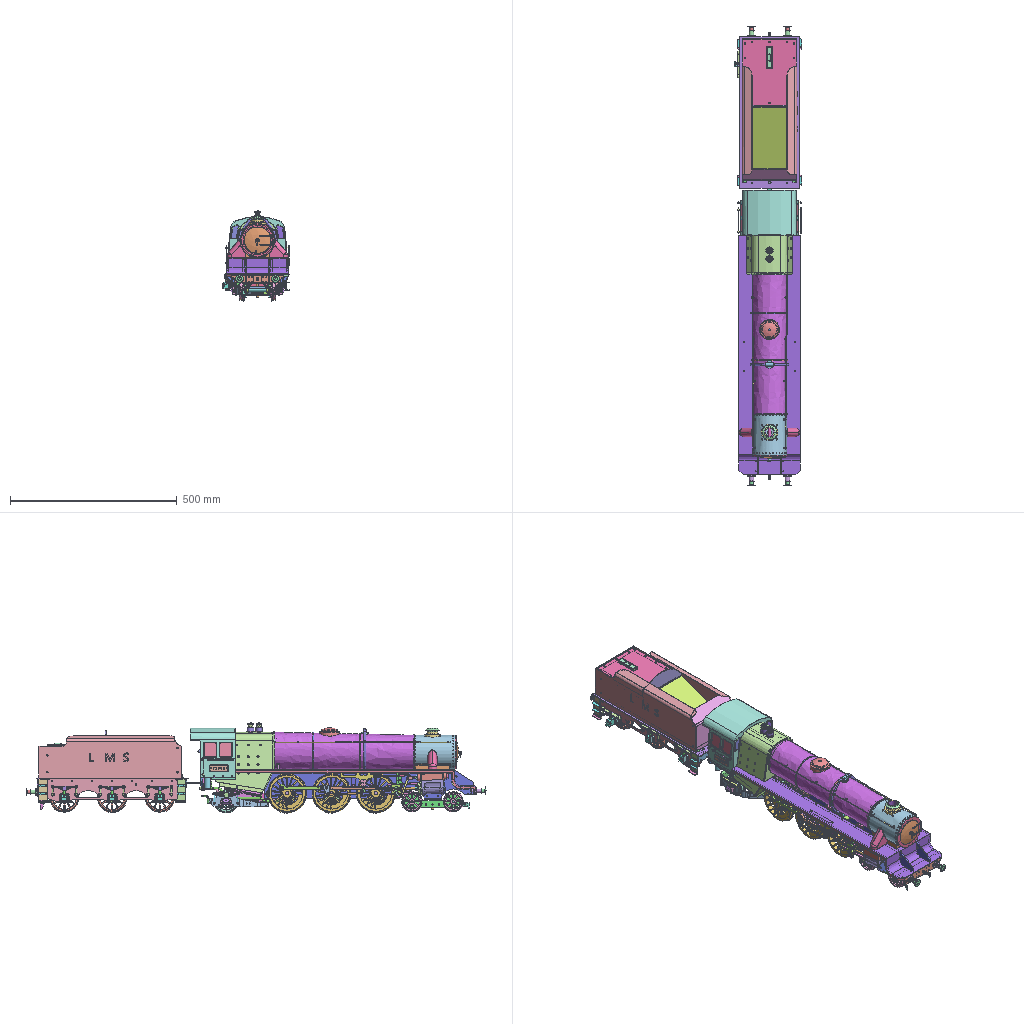Assembly | STEP file | 318 different items | 619 placed | box 202 x 1378 x 271 mm
Parts list (item | name | quantity | parent item | size | volume):
1 | 1-01.14 | x1 | in 1-01 part | 10 x 10 x 33 mm | 1037 mm3
2 | 1-01.13 | x2 | in 1-01 part | 26 x 12 x 30 mm | 2499 mm3
3 | 1-01.12 | x1 | in 1-01 part | 13 x 67 x 13 mm | 5525 mm3
4 | 1-01.11 | x1 | in 1-01 part | 20 x 20 x 1 mm | 235.619 mm3
5 | 1-01.10 | x1 | in 1-01 part | 14.501 x 14.501 x 19.996 mm | 434.428 mm3
6 | 1-01.9 | x1 | in 1-01 part | 10 x 10 x 41 mm | 2711 mm3
7 | 1-01.8 | x2 | in 1-01 part | 51 x 12 x 12 mm | 2118 mm3
8 | 1-01.7 | x1 | in 1-01 part | 51 x 73 x 3 mm | 10792 mm3
9 | 1-01.6 | x1 | in 1-01 part | 16 x 67 x 38 mm | 16896 mm3
10 | 1-01.5 | x2 | in 1-01 part | 21 x 21 x 21 mm | 2287 mm3
11 | 1-01.4 symmetric part | x1 | in 1-01 part | 577.1 x 8 x 56 mm | 13016 mm3
12 | 1-01.4 | x1 | in 1-01 part | 577.1 x 8 x 56 mm | 13016 mm3
13 | 1-01.3 | x1 | in 1-01 part | 12 x 67 x 25 mm | 18121 mm3
14 | 1-01.2 | x1 | in 1-01 part | 25 x 152 x 25 mm | 25515 mm3
15 | 1-01.1 | x2 | in 1-01 part | 3 x 625 x 82.5 mm | 131350 mm3
16 | 1-02 | x6 | in Locomotive assembly | 13 x 50 x 13 mm | 2573 mm3
17 | 1-03.1 | x6 | in 1-03 part | 10 x 25 x 25 mm | 4620 mm3
18 | 1-03.2 | x6 | in 1-03 part | 3 x 3 x 39 mm | 275.675 mm3
19 | 1-03.3 | x6 | in 1-03 part | 5.252 x 5.25 x 22.544 mm | 75.49 mm3
20 | 1-03.4 | x6 | in 1-03 part | 6 x 6 x 1 mm | 21.206 mm3
21 | 1-04.1 | x2 | in 1-04 part | 3 x 173.195 x 38 mm | 12978 mm3
22 | 1-04.2 | x1 | in 1-04 part | 50 x 68 x 12 mm | 11705 mm3
23 | 1-04.3 | x2 | in 1-04 part | 7 x 68 x 7 mm | 2391 mm3
24 | 1-04.4 | x4 | in 1-04 part | 19 x 13 x 19 mm | 1368 mm3
25 | 1-04.5 | x1 | in 1-04 part | 11 x 30 x 17.5 mm | 723.407 mm3
26 | 1-04.5 symmetric part | x1 | in 1-04 part | 11 x 30 x 17.5 mm | 723.407 mm3
27 | 1-05 | x1 | in Locomotive assembly | 106 x 78.066 x 28.5 mm | 78441 mm3
28 | 1-06.1 | x2 | in 1-06 part, 1-06 symmetric subassembly | 64 x 54.5 x 45 mm | 79802 mm3
29 | 1-06.2 | x2 | in 1-06 part, 1-06 symmetric subassembly | 28 x 64 x 28 mm | 7900 mm3
30 | 1-06.3 | x2 | in 1-06 part, 1-06 symmetric subassembly | 13.856 x 12 x 12 mm | 1127 mm3
31 | 1-06.4 | x2 | in 1-06 part, 1-06 symmetric subassembly | 13.856 x 11.5 x 12 mm | 920.282 mm3
32 | 1-06.5 | x2 | in 1-06 part, 1-06 symmetric subassembly | 8 x 4.5 x 8 mm | 169.646 mm3
33 | 1-06.6 | x2 | in 1-06 part, 1-06 symmetric subassembly | 8 x 5.5 x 8 mm | 119.381 mm3
34 | 1-06.7 | x2 | in 1-06 part, 1-06 symmetric subassembly | 45 x 64 x 3 mm | 8287 mm3
35 | 1-06.8 | x2 | in 1-06 part, 1-06 symmetric subassembly | 54.5 x 88 x 23 mm | 33301 mm3
36 | 1-07 | x2 | in Locomotive assembly | 6.5 x 45 x 45 mm | 8285 mm3
37 | 1-08.1 | x2 | in 1-08 part | 13.5 x 45 x 45 mm | 10498 mm3
38 | 1-08.2 | x4 | in 1-08 part | 101 x 6 x 5 mm | 2812 mm3
39 | 1-08.3 | x2 | in 1-08 part | 13.5 x 18.475 x 16 mm | 1580 mm3
40 | 1-08.4 | x2 | in 1-08 part | 4 x 10 x 10 mm | 201.062 mm3
41 | 1-08.5 | x2 | in 1-08 part | 4 x 10 x 10 mm | 144.513 mm3
42 | 1-09.1 | x1 | in Locomotive assembly | 24 x 38 x 77 mm | 9451 mm3
43 | 1-09.1 symmetric part | x1 | in Locomotive assembly | 24 x 38 x 77 mm | 9451 mm3
44 | 1-11.1 | x1 | in 1-11 part | 25 x 40 x 48 mm | 7483 mm3
45 | 1-11.2 | x1 | in 1-11 part | 15 x 17.321 x 16 mm | 1681 mm3
46 | 1-11.3 | x2 | in 1-11 part | 8 x 38 x 8 mm | 835.664 mm3
47 | 1-11.4 | x2 | in 1-11 part | 13.856 x 4 x 12 mm | 297.769 mm3
48 | 1-12.1 | x1 | in 1-12 part | 25 x 14 x 70 mm | 4367 mm3
49 | 1-12.2 | x2 | in 1-12 part | 38 x 10 x 10 mm | 1074 mm3
50 | 1-12.3 | x2 | in 1-12 part | 4 x 16.166 x 14 mm | 364.805 mm3
51 | 1-12.4 | x1 | in 1-12 part | 10 x 11.547 x 13 mm | 537.367 mm3
52 | 1-14.1 | x1 | in 1-14 part | 50.002 x 50.001 x 27 mm | 7555 mm3
53 | 1-14.2 | x1 | in 1-14 part | 36 x 36 x 64.039 mm | 7996 mm3
54 | 1-14.3 | x1 | in 1-14 part | 44 x 44 x 9.5 mm | 3548 mm3
55 | 1-15 | x1 | in Locomotive assembly | 60.001 x 60 x 25.516 mm | 4981 mm3
56 | 1-16.1 | x2 | in 1-16 part | 12 x 12 x 4 mm | 306.305 mm3
57 | 1-16.2 | x2 | in 1-16 part | 16 x 16 x 19 mm | 1038 mm3
58 | 1-16.3 | x2 | in 1-16 part | 4.501 x 4.5 x 11.798 mm | 24.723 mm3
59 | 1-16.4 | x2 | in 1-16 part | 6 x 6 x 20 mm | 175.087 mm3
60 | 1-16.5 | x2 | in 1-16 part | 6 x 6 x 6 mm | 113.097 mm3
61 | 1-16.6 | x2 | in 1-16 part | 19 x 19 x 20 mm | 2980 mm3
62 | 1-23.1 | x1 | in 1-23 part | 37 x 32 x 32 mm | 6942 mm3
63 | 1-23.2 | x1 | in 1-23 part | 142 x 14 x 14 mm | 14676 mm3
64 | 1-23.3 | x1 | in 1-23 part | 21 x 14 x 14 mm | 1943 mm3
65 | 1-23.4 | x1 | in 1-23 part | 427 x 10 x 10 mm | 20870 mm3
66 | 1-23.5 | x1 | in 1-23 part | 185.5 x 10 x 10 mm | 6004 mm3
67 | 1-23.6 | x1 | in 1-23 part | 14 x 17.321 x 15 mm | 1648 mm3
68 | 1-23.7 | x1 | in 1-23 part | 24.52 x 10 x 38.054 mm | 795.308 mm3
69 | 1-26.1 | x1 | in 1-26 part | 8 x 315 x 31 mm | 5686 mm3
70 | 1-26.2 | x1 | in 1-26 part | 8 x 392.074 x 38.526 mm | 7072 mm3
71 | 1-26.3 | x1 | in 1-26 part | 7 x 12 x 22 mm | 969.173 mm3
72 | 1-26.4 | x1 | in 1-26 part | 3 x 12 x 22 mm | 652.172 mm3
73 | 1-28.1 | x1 | in 1-28 part | 184 x 821 x 50 mm | 191096 mm3
74 | 1-28.2 | x1 | in 1-28 part | 716 x 16 x 54 mm | 8341 mm3
75 | 1-28.2 symmetric part | x1 | in 1-28 part | 716 x 16 x 54 mm | 8341 mm3
76 | 1-28.3 | x1 | in 1-28 part | 5 x 172 x 24 mm | 17032 mm3
77 | 1-28.4 | x1 | in 1-28 part | 22 x 110 x 15 mm | 4787 mm3
78 | 1-28.5 | x2 | in 1-28 part | 32 x 5 x 20.5 mm | 1373 mm3
79 | 1-28.6 | x1 | in 1-28 part | 10 x 80 x 3 mm | 2218 mm3
80 | 1-28.7 | x6 | in 1-28 part | 12.702 x 3 x 11 mm | 163.571 mm3
81 | 1-28.8 | x3 | in 1-28 part | 8 x 10 x 8 mm | 219.911 mm3
82 | 1-28.9 | x1 | in 1-28 part | 8 x 8 x 27 mm | 568.112 mm3
83 | 1-28.10 | x2 | in Locomotive assembly | 13 x 100 x 46.631 mm | 6044 mm3
84 | 1-29.1 | x2 | in 1-29 part | 31 x 23 x 23 mm | 3301 mm3
85 | 1-29.2 | x2 | in 1-29 part | 46.201 x 23 x 23 mm | 2003 mm3
86 | 1-29.3 | x2 | in 1-29 part | 13.747 x 6.8 x 6.802 mm | 67.319 mm3
87 | 1-30.1 | x2 | in 1-30 part | 4 x 31.452 x 9.916 mm | 569.945 mm3
88 | 1-30.2 | x2 | in 1-30 part | 8.998 x 7.25 x 7.252 mm | 54.263 mm3
89 | 1-30.3 | x2 | in 1-30 part | 1 x 8 x 8 mm | 43.197 mm3
90 | 1-31.1 | x1 | in 1-31 part | 135 x 172 x 146.5 mm | 47379 mm3
91 | 1-31.2 | x1 | in 1-31 part | 10 x 102 x 6 mm | 1488 mm3
92 | 1-31.4 | x1 | in 1-31 part | 1 x 20.769 x 39.162 mm | 584.948 mm3
93 | 1-31.5 | x1 | in 1-31 part | 2 x 24.769 x 43.162 mm | 321.973 mm3
94 | 1-31.6 | x4 | in 1-31 part | 1 x 36 x 42 mm | 1498 mm3
95 | 1-31.7 | x4 | in 1-31 part | 3 x 40 x 46 mm | 615.381 mm3
96 | 1-33.1 | x8 | in 1-31 part | 6 x 6 x 14 mm | 146.542 mm3
97 | 1-33.2 | x2 | in 1-31 part | 80 x 2 x 2 mm | 251.327 mm3
98 | 1-34 | x2 | in 1-31 part | 58 x 2 x 2 mm | 182.212 mm3
99 | 1-38 | x2 | in 1-31 part | 1.5 x 57 x 21 mm | 1289 mm3
100 | 1-31.4 symmetric part | x1 | in 1-31 part | 1 x 20.769 x 39.162 mm | 584.948 mm3
101 | 1-31.5 symmetric part | x1 | in 1-31 part | 2 x 24.769 x 43.162 mm | 321.973 mm3
102 | 1-46.1 | x1 | in Locomotive assembly | 38 x 82 x 50 mm | 26296 mm3
103 | 1-46.2 | x1 | in Locomotive assembly | 76 x 24 x 24 mm | 12833 mm3
104 | 1-46.3 | x1 | in Locomotive assembly | 13 x 19 x 19 mm | 2578 mm3
105 | 1-46.4 | x1 | in Locomotive assembly | 32 x 16 x 50 mm | 9921 mm3
106 | 1-46.5 | x1 | in Locomotive assembly | 15 x 17.321 x 12 mm | 1383 mm3
107 | 1-46.6 | x2 | in Locomotive assembly | 7 x 7 x 7 mm | 179.594 mm3
108 | 1-46.7 | x1 | in Locomotive assembly | 15 x 17.321 x 18 mm | 2228 mm3
109 | 1-46.8 | x1 | in Locomotive assembly | 14 x 16.166 x 14 mm | 1298 mm3
110 | 1-46.9 | x1 | in Locomotive assembly | 6 x 12 x 28 mm | 1411 mm3
111 | 1-46.10 | x2 | in Locomotive assembly | 3 x 88 x 12 mm | 3000 mm3
112 | 1-46.11 | x1 | in Locomotive assembly | 19 x 91.264 x 19 mm | 21626 mm3
113 | 1-46.12 | x1 | in Locomotive assembly | 19.5 x 10 x 19.5 mm | 1406 mm3
114 | 1-46.13 | x1 | in Locomotive assembly | 20 x 11 x 65.5 mm | 4616 mm3
115 | 1-51.1 | x1 | in 1-51 part | 16 x 30 x 41 mm | 5743 mm3
116 | 1-51.2 | x2 | in 1-51 part | 13 x 15.011 x 12 mm | 1011 mm3
117 | 1-51.4 | x1 | in 1-51 part | 13 x 15.011 x 4 mm | 263.292 mm3
118 | 1-51.3 | x1 | in Locomotive assembly | 6 x 48 x 47.5 mm | 691.647 mm3
119 | 1-51.6 | x1 | in Locomotive assembly | 6 x 175 x 42.678 mm | 1626 mm3
120 | 1-53.1 | x1 | in 1-53 part | 50.5 x 178 x 44 mm | 13131 mm3
121 | 1-53.2 | x4 | in 1-53 part | 12 x 10 x 22 mm | 987.448 mm3
122 | 1-53.3 | x2 | in 1-53 part | 2 x 46 x 8.5 mm | 425.407 mm3
123 | 1-53.4 | x4 | in 1-53 part | 17 x 8 x 4 mm | 352.221 mm3
124 | 1-53.5 | x1 | in 1-53 part | 12 x 25 x 12 mm | 3063 mm3
125 | 1-53.6 | x1 | in 1-53 part | 36 x 120 x 24 mm | 15140 mm3
126 | 1-53.7 | x1 | in 1-53 part | 18 x 104.1 x 16 mm | 6325 mm3
127 | 1-53.1 symmetric part | x1 | in 1-53 part | 50.5 x 178 x 44 mm | 13131 mm3
128 | 1-54.1 | x2 | in 1-54 part | 8 x 80 x 10 mm | 4102 mm3
129 | 1-54.2 | x2 | in 1-54 part | 12 x 11 x 13 mm | 718.301 mm3
130 | 1-54.3 | x2 | in 1-54 part | 7 x 7 x 22.5 mm | 528.966 mm3
131 | 1-54.4 | x4 | in 1-54 part | 6 x 6 x 34 mm | 281.77 mm3
132 | 1-54.5 | x2 | in 1-54 part | 9 x 15 x 9 mm | 530.144 mm3
133 | 1-54.6 | x2 | in 1-54 part | 16 x 22 x 16 mm | 3574 mm3
134 | 1-55.1 | x1 | in 1-55 part | 44 x 16 x 44 mm | 8886 mm3
135 | 1-55.2 | x1 | in 1-55 part | 16 x 36 x 33 mm | 3784 mm3
136 | 1-55.3 | x1 | in 1-55 part | 16 x 30 x 23 mm | 3666 mm3
137 | 1-55.4 | x1 | in 1-55 part | 6 x 6 x 6 mm | 113.097 mm3
138 | 1-55.5 | x3 | in 1-55 part | 12.5 x 15.011 x 13 mm | 1071 mm3
139 | 1-55.6 | x1 | in 1-55 part | 24.249 x 8 x 21 mm | 1799 mm3
140 | 1-55.7 | x1 | in 1-55 part | 20.785 x 18 x 18 mm | 3019 mm3
141 | 1-56.1 | x1 | in Locomotive assembly | 102 x 13 x 102 mm | 22776 mm3
142 | 1-56.2 | x1 | in Locomotive assembly | 102 x 122 x 102 mm | 92054 mm3
143 | 1-56.3 | x1 | in Locomotive assembly | 97 x 20 x 97 mm | 24368 mm3
144 | 1-56.4 | x1 | in Locomotive assembly | 102.005 x 421.966 x 111 mm | 341502 mm3
145 | 1-56.5 | x1 | in Locomotive assembly | 22 x 22 x 7 mm | 989.602 mm3
146 | 1-56.6 | x1 | in Locomotive assembly | 28 x 28 x 9 mm | 2554 mm3
147 | 1-56.7 | x1 | in Locomotive assembly | 22 x 25.403 x 21 mm | 4474 mm3
148 | 1-56.8 | x1 | in Locomotive assembly | 157.85 x 175.6 x 171.3 mm | 188162 mm3
149 | 1-56.9 | x2 | in Locomotive assembly | 22 x 22 x 8 mm | 1653 mm3
150 | 1-56.10 | x1 | in Locomotive assembly | 144.937 x 39.504 x 145.902 mm | 83548 mm3
151 | 1-56.11 | x1 | in Locomotive assembly | 152.783 x 146.73 x 32.367 mm | 19340 mm3
152 | 1-56.12 | x1 | in Locomotive assembly | 10 x 97 x 106 mm | 9399 mm3
153 | 1-56.13 | x1 | in Locomotive assembly | 17 x 32 x 32 mm | 4706 mm3
154 | 1-56.14 | x1 | in Locomotive assembly | 35 x 36 x 20 mm | 6413 mm3
155 | 1-56.15 | x1 | in Locomotive assembly | 12 x 36 x 20 mm | 5657 mm3
156 | 1-56.16 | x1 | in Locomotive assembly | 32 x 290 x 32 mm | 54664 mm3
157 | 1-56.17 | x4 | in Locomotive assembly | 19 x 290 x 19 mm | 12470 mm3
158 | 1-56.18 | x1 | in Locomotive assembly | 165.767 x 74.2 x 6 mm | 18558 mm3
159 | 1-56.19 | x1 | in Locomotive assembly | 86.75 x 10.5 x 80 mm | 24295 mm3
160 | 1-56.20 | x2 | in Locomotive assembly | 4 x 8 x 4 mm | 81.772 mm3
161 | 1-56.21 | x1 | in Locomotive assembly | 3 x 3 x 33 mm | 107.521 mm3
162 | 1-56.22 | x2 | in Locomotive assembly | 28 x 54 x 60.117 mm | 6024 mm3
163 | 1-56.23 | x10 | in Locomotive assembly | 12 x 4 x 4 mm | 60.89 mm3
164 | 1-56.24 | x2 | in Locomotive assembly | 5.973 x 524.553 x 2 mm | 1650 mm3
165 | 1-56.25 | x1 | in Locomotive assembly | 105 x 3 x 105 mm | 1463 mm3
166 | 1-56.26 | x1 | in Locomotive assembly | 105 x 3 x 114.181 mm | 1546 mm3
167 | 1-56.27 | x1 | in Locomotive assembly | 3 x 108 x 108.5 mm | 1510 mm3
168 | 1-56.28 | x1 | in Locomotive assembly | 3 x 110 x 112 mm | 1552 mm3
169 | 1-57.1 | x1 | in 1-57 part | 288.5 x 140.126 x 141.936 mm | 221240 mm3
170 | 1-57.2 | x1 | in 1-57 part | 12 x 90.4 x 70.538 mm | 15171 mm3
171 | 1-57.3 | x2 | in 1-57 part | 19.001 x 19.001 x 66.2 mm | 3399 mm3
172 | 1-57.4 | x1 | in 1-57 part | 12.749 x 134.024 x 120.156 mm | 31818 mm3
173 | 1-57.5 | x1 | in 1-57 part | 33.418 x 126.49 x 118.588 mm | 41627 mm3
174 | 1-57.6 | x1 | in Locomotive assembly | 19.684 x 150 x 44.877 mm | 17988 mm3
175 | 1-57.6 symmetric part | x1 | in Locomotive assembly | 19.684 x 150 x 44.877 mm | 17988 mm3
176 | 1-58A | x1 | in Locomotive assembly | 18 x 18 x 11 mm | 1131 mm3
177 | 1-58B | x1 | in Locomotive assembly | 20 x 20 x 11 mm | 1307 mm3
178 | 1-59 | x1 | in Locomotive assembly | 77.36 x 10 x 46.251 mm | 6866 mm3
179 | 1-60U | x1 | in Locomotive assembly | 11 x 18 x 18 mm | 1131 mm3
180 | 1-60L | x1 | in Locomotive assembly | 21 x 18 x 18 mm | 1885 mm3
181 | 1-61.1 | x1 | in 1-61 part | 15.011 x 17 x 13 mm | 1376 mm3
182 | 1-61.2 | x1 | in 1-61 part | 17 x 25 x 17 mm | 1909 mm3
183 | 1-62 | x1 | in Locomotive assembly | 23.5 x 54 x 42 mm | 8085 mm3
184 | 1-63 | x1 | in Locomotive assembly | 8 x 54 x 42 mm | 12146 mm3
185 | 1-63.2 | x2 | in Locomotive assembly | 5 x 29 x 5 mm | 183.888 mm3
186 | 1-63.3 | x1 | in Locomotive assembly | 10.75 x 3.5 x 24 mm | 107.386 mm3
187 | 1-63.4 | x1 | in Locomotive assembly | 4.5 x 4.5 x 26 mm | 106.486 mm3
188 | 1-63.5 | x1 | in Locomotive assembly | 5 x 20 x 4 mm | 81.74 mm3
189 | 1-63.6 | x1 | in Locomotive assembly | 7 x 4 x 4 mm | 61.425 mm3
190 | 1-64 | x24 | in Locomotive assembly | 17.557 x 6.3 x 6.3 mm | 224.928 mm3
191 | 1-65.1 | x2 | in Locomotive assembly | 15 x 29 x 21.57 mm | 2510 mm3
192 | 1-65.2 | x2 | in Locomotive assembly | 12 x 13.856 x 8 mm | 766.822 mm3
193 | 1-65.3 | x2 | in Locomotive assembly | 12 x 12 x 2 mm | 98.696 mm3
194 | 1-65.4 | x1 | in Locomotive assembly | 8 x 8 x 40 mm | 1225 mm3
195 | 1-65.5 | x2 | in Locomotive assembly | 15 x 17.321 x 10 mm | 938.524 mm3
196 | 1-67.1 | x1 | in 1-67 part | 25 x 22 x 32.5 mm | 4130 mm3
197 | 1-67.2 | x1 | in 1-67 part | 5.501 x 5.5 x 9.499 mm | 30.865 mm3
198 | 1-67.3 | x1 | in 1-67 part | 6 x 6 x 6 mm | 113.097 mm3
199 | 1-67.4 | x1 | in 1-67 part | 10 x 10 x 9 mm | 482.855 mm3
200 | 1-63 part screw | x4 | in Locomotive assembly | 6.956 x 4.807 x 4.807 mm | 51.542 mm3
201 | 1-63部分2毫米Bolt | x1 | in Locomotive assembly | 4.5 x 2.646 x 2.646 mm | 14.006 mm3
202 | 1-68.1 | x1 | in 1-68 part | 122 x 13.367 x 34.723 mm | 14145 mm3
203 | 1-68.2 | x1 | in 1-68 part | 8 x 52 x 20 mm | 7189 mm3
204 | 1-69.9 | x1 | in 1-69 part | 148 x 5 x 5 mm | 2906 mm3
205 | 1-69.8 | x2 | in 1-69 part | 116 x 5 x 5 mm | 2278 mm3
206 | 1-69.6 | x1 | in 1-69 part | 24 x 56 x 11 mm | 3285 mm3
207 | 1-69.5 | x4 | in 1-69 part | 6 x 9 x 39.5 mm | 1888 mm3
208 | 1-69.4 | x10 | in 1-69 part | 6 x 122 x 12 mm | 8548 mm3
209 | 1-69.3 | x8 | in 1-69 part | 9 x 6 x 9 mm | 263.894 mm3
210 | 1-69.2 | x2 | in 1-69 part | 9 x 4 x 9 mm | 175.929 mm3
211 | 1-69.1 | x1 | in 1-69 part | 107.541 x 129.236 x 49 mm | 41609 mm3
212 | 1-70.1 | x1 | in Locomotive assembly | 28 x 18.5 x 9 mm | 1316 mm3
213 | 1-70.2 | x1 | in Locomotive assembly | 6 x 192.5 x 24 mm | 1698 mm3
214 | 1-70.3 | x2 | in Locomotive assembly | 6 x 54 x 128 mm | 1514 mm3
215 | 1-71 | x1 | in Locomotive assembly | 62.108 x 259 x 78 mm | 3437 mm3
216 | 1-72 | x1 | in Locomotive assembly | 24 x 279.352 x 42 mm | 2708 mm3
217 | 1-73.1 | x1 | in 1-73 | 24 x 16 x 42.5 mm | 6373 mm3
218 | 1-73.2 | x1 | in 1-73 | 14 x 16.166 x 3 mm | 263.877 mm3
219 | 1-73.3 | x1 | in 1-73 | 14 x 16.166 x 10 mm | 1039 mm3
220 | 1-73.4 | x1 | in 1-73 | 10 x 10 x 6 mm | 194.779 mm3
221 | 1-73.7 | x1 | in Locomotive assembly | 6 x 40 x 6 mm | 345.575 mm3
222 | 1-73.8 | x1 | in Locomotive assembly | 9 x 9 x 17 mm | 786.768 mm3
223 | 1-73.9 | x1 | in Locomotive assembly | 6 x 22 x 6 mm | 190.066 mm3
224 | 1-73.5 | x1 | in Locomotive assembly | 6 x 6 x 75.5 mm | 1086 mm3
225 | 1-73.6 | x1 | in Locomotive assembly | 22 x 22 x 3.5 mm | 1272 mm3
226 | 1-74 | x1 | in Locomotive assembly | 6 x 253 x 126 mm | 3148 mm3
227 | 1-75.1 | x1 | in 1-75 part | 41 x 29 x 30 mm | 6004 mm3
228 | 1-75.2 | x2 | in 1-75 part | 13 x 15.011 x 3 mm | 194.333 mm3
229 | 1-75.3 | x1 | in 1-75 part | 12 x 11.547 x 10 mm | 521.946 mm3
230 | 1-75.4 | x1 | in 1-75 part | 17 x 13.856 x 12 mm | 858.508 mm3
231 | 1-75.5 | x1 | in 1-75 part | 11 x 13.856 x 12 mm | 966.779 mm3
232 | 1-75.6 | x1 | in Locomotive assembly | 57 x 8 x 8 mm | 1037 mm3
233 | 1-75.7 | x1 | in Locomotive assembly | 3 x 22 x 22 mm | 1050 mm3
234 | 1-75.8 | x1 | in Locomotive assembly | 6 x 112.85 x 19.5 mm | 1008 mm3
235 | 2-04.1 | x4 | in 2-04 part | 63 x 17 x 63 mm | 20551 mm3
236 | 2-04.2 | x2 | in 2-04 part | 12 x 115 x 12 mm | 10469 mm3
237 | 2-01.1 | x6 | in 2-01 part, 2-02 part, 2-03 part | 120 x 17 x 120 mm | 77367 mm3
238 | 2-01.2 | x3 | in 2-01 part, 2-02 part, 2-03 part | 12 x 115 x 12 mm | 11831 mm3
239 | 2-01.3 | x2 | in 2-01 part | 7 x 38 x 7 mm | 1195 mm3
240 | COMPOUND | x2 | in 2-01.4 | 7 x 17 x 32.5 mm | 1174 mm3
241 | COMPOUND | x2 | in 2-01.4 | - | -
242 | 2-02.3 | x2 | in 2-02 part | 23 x 11 x 11 mm | 853.955 mm3
243 | 2-03.3 | x2 | in 2-03 part | 29 x 7 x 7 mm | 829.38 mm3
244 | 2-14.1 | x2 | in 2-14 part | 70 x 17 x 70 mm | 25779 mm3
245 | 2-14.2 | x1 | in 2-14 part | 10 x 145 x 10 mm | 8902 mm3
246 | COMPOUND | x1 | in 2-05.1 | 6 x 163 x 19 mm | 7089 mm3
247 | COMPOUND | x1 | in 2-05.1 | - | -
248 | 2-05.1 symmetric part | x1 | in Locomotive assembly | 6 x 163 x 19 mm | 7089 mm3
249 | 2-05.2 | x1 | in Locomotive assembly | 6 x 131 x 19 mm | 5279 mm3
250 | 2-05.2 symmetric part | x1 | in Locomotive assembly | 6 x 131 x 19 mm | 5279 mm3
251 | 2-06.1 | x2 | in 2-06 part, 2-06 symmetric subassembly | 13 x 25 x 25 mm | 5232 mm3
252 | 2-06.2 | x2 | in 2-06 part, 2-06 symmetric subassembly | 25.2 x 5 x 25.2 mm | 921.7 mm3
253 | 2-06.3 | x2 | in 2-06 part, 2-06 symmetric subassembly | 6 x 89 x 10 mm | 2444 mm3
254 | 2-06.4 | x1 | in 2-06 part | 13 x 30 x 27.66 mm | 5154 mm3
255 | 2-06.5 | x2 | in 2-06 part, 2-06 symmetric subassembly | 14 x 16 x 14 mm | 769.46 mm3
256 | 2-07 | x1 | in Locomotive assembly | 10 x 225 x 23.5 mm | 9355 mm3
257 | 2-07 symmetric part | x1 | in Locomotive assembly | 10 x 225 x 23.5 mm | 9355 mm3
258 | 2-09.1 | x2 | in 2-09 | 3 x 12 x 35.5 mm | 947.961 mm3
259 | 2-09.2 | x2 | in 2-09 | 5 x 12 x 5 mm | 122.522 mm3
260 | 2-09.3 | x2 | in 2-09 | 38 x 6 x 12 mm | 1105 mm3
261 | 2-09.4 | x2 | in 2-09 | 9 x 12.001 x 29.5 mm | 1794 mm3
262 | 2-09.5 | x2 | in 2-09 | 8 x 11 x 8 mm | 231.567 mm3
263 | 2-11.1 | x2 | in 2-11 part, 2-11 symmetric subassembly | 19 x 24 x 14.792 mm | 4772 mm3
264 | 2-11.2 | x2 | in 2-11 part, 2-11 symmetric subassembly | 5 x 86 x 5 mm | 1019 mm3
265 | 2-11.3 | x2 | in 2-11 part, 2-11 symmetric subassembly | 9 x 21.5 x 9 mm | 963.016 mm3
266 | 2-11.4 | x2 | in 2-11 part, 2-11 symmetric subassembly | 17 x 4 x 4 mm | 169.646 mm3
267 | 2-06.4 symmetric part | x1 | in 2-06 symmetric subassembly | 13 x 30 x 27.66 mm | 5154 mm3
268 | 1-35.2 | x1 | in 1-35 | 4 x 5.337 x 12.426 mm | 50.541 mm3
269 | 1-35.1 | x1 | in 1-35 | 7 x 18.051 x 47 mm | 449.87 mm3
270 | 2-13 | x2 | in Locomotive assembly | 6.5 x 108 x 10 mm | 1291 mm3
271 | 2-14 | x2 | in Locomotive assembly | 16 x 13.946 x 58.697 mm | 1069 mm3
272 | 2-17 | x2 | in Locomotive assembly | 5 x 165 x 5 mm | 803.778 mm3
273 | 2-19 | x2 | in Locomotive assembly | 8 x 10.503 x 19.146 mm | 448.562 mm3
274 | 2-18 | x2 | in Locomotive assembly | 11 x 6 x 72 mm | 957.208 mm3
275 | 2-20 | x2 | in Locomotive assembly | 5 x 21 x 6 mm | 222.849 mm3
276 | 1-43.11 | x1 | in Locomotive assembly | 64 x 16 x 11 mm | 1944 mm3
277 | 2-13.1 | x6 | in 2-13 part | 91 x 17 x 91 mm | 34927 mm3
278 | 2-13.2 | x3 | in 2-13 part | 10 x 145 x 10 mm | 8915 mm3
279 | 1-47.1 | x2 | in 1-47 | 15 x 30 x 70 mm | 3583 mm3
280 | 1-47.2 | x4 | in 1-47, 1-47 symmetric subassembly | 10.5 x 30 x 6 mm | 658.288 mm3
281 | 1-47.3 | x8 | in 1-47, 1-47 symmetric subassembly | 10 x 24 x 6 mm | 510 mm3
282 | 1-47.1 symmetric part | x2 | in 1-47 symmetric subassembly | 15 x 30 x 70 mm | 3583 mm3
283 | 1-43.1 | x1 | in Tender assembly | 178 x 454 x 2.5 mm | 200860 mm3
284 | 1-43.2 | x1 | in Tender assembly | 427 x 160 x 10 mm | 35939 mm3
285 | 1-43.3 | x1 | in Tender assembly | 427 x 165 x 126.605 mm | 256385 mm3
286 | 1-43.4 | x1 | in Tender assembly | 200 x 160 x 12 mm | 42705 mm3
287 | 1-43.5 | x1 | in Tender assembly | 160 x 233 x 13.692 mm | 58766 mm3
288 | 1-43.6 | x1 | in Tender assembly | 160 x 34.183 x 126.611 mm | 40223 mm3
289 | 1-43.7 | x1 | in Tender assembly | 10 x 156 x 10 mm | 5296 mm3
290 | 1-43.8 | x1 | in Tender assembly | 20 x 96 x 38 mm | 14395 mm3
291 | 1-43.9 | x1 | in Tender assembly | 3 x 160 x 51.122 mm | 19342 mm3
292 | 1-43.10 | x1 | in Tender assembly | 66 x 18 x 9 mm | 1568 mm3
293 | 1-43.12 | x1 | in Tender assembly | 197 x 160 x 1.5 mm | 45442 mm3
294 | 1-43.14 | x3 | in Tender assembly | 19 x 8 x 8 mm | 417.832 mm3
295 | 1-43.15 | x6 | in Tender assembly | 3 x 11.547 x 10 mm | 106.106 mm3
296 | 1-41.1 | x6 | in 1-41 part | 10 x 79 x 29.5 mm | 5148 mm3
297 | 1-41.2 | x12 | in 1-41 part | 9.5 x 9 x 8.5 mm | 174.881 mm3
298 | 1-41.3 | x6 | in 1-41 part | 15 x 23.5 x 20 mm | 4873 mm3
299 | 1-41.4 | x6 | in 1-41 part | 8 x 15.5 x 8 mm | 340.863 mm3
300 | 1-41.5 | x6 | in 1-41 part | 10 x 11 x 12 mm | 305.863 mm3
301 | 1-41.6 | x6 | in 1-41 part | 6 x 6 x 26 mm | 478.438 mm3
302 | 1-40.1 | x2 | in 1-40 part | 3 x 438 x 70 mm | 72359 mm3
303 | 1-40.2 | x1 | in 1-40 part | 25 x 172 x 25 mm | 31997 mm3
304 | 1-40.3 | x1 | in 1-40 part | 20 x 20 x 45.5 mm | 5971 mm3
305 | 1-40.3 symmetric part | x1 | in 1-40 part | 20 x 20 x 45.5 mm | 5971 mm3
306 | 1-40.4 | x1 | in 1-40 part | 20 x 20 x 20 mm | 2622 mm3
307 | 1-40.4 symmetric part | x1 | in 1-40 part | 20 x 20 x 20 mm | 2622 mm3
308 | 1-40.5 | x1 | in 1-40 part | 9 x 9 x 27.5 mm | 617.052 mm3
309 | 1-40.7 | x6 | in 1-40 part | 3 x 33 x 5 mm | 291.958 mm3
310 | 1-40.8 | x1 | in 1-40 part | 13 x 24 x 9.5 mm | 924.566 mm3
311 | 1-40.9 | x12 | in 1-40 part | 9 x 14 x 23.6 mm | 1143 mm3
312 | 1-40.10 | x2 | in 1-40 part | 12 x 398 x 12 mm | 17261 mm3
313 | 1-40.11 | x1 | in 1-40 part | 25 x 172 x 51.75 mm | 54650 mm3
314 | 1-42.1 | x2 | in 1-42 part | 26 x 23 x 23 mm | 2672 mm3
315 | 1-42.2 | x2 | in 1-42 part | 37.201 x 23 x 23 mm | 1939 mm3
316 | 1-42.3 | x2 | in 1-42 part | 13.747 x 6.8 x 6.802 mm | 67.319 mm3
317 | 1-50 | x1 | in Tender assembly | 17 x 20 x 54 mm | 1793 mm3
318 | 1-50 symmetric part | x1 | in Tender assembly | 17 x 20 x 54 mm | 1793 mm3
Placements (level | parent | child | x y z in mm | rotation matrix by rows), first 267 of 689 lines:
1 | Locomotive assembly | 1-01 part | 0.0 0.0 0.0 | 1 0 0 0 1 0 0 0 1
2 | 1-01 part | 1-01.14 | 36.5 559.0 0.0 | -0.9037 0.4281 0 -0.4281 -0.9037 0 0 0 1
2 | 1-01 part | 1-01.13 | 3.0 298.5 38.0 | 1 0 0 0 1 0 0 0 1
2 | 1-01 part | 1-01.13 | 70.0 298.5 38.0 | -1 0 0 0 1 0 0 0 -1
2 | 1-01 part | 1-01.12 | 36.5 257.0 57.5 | 0 1 0 -1 0 0 0 0 1
2 | 1-01 part | 1-01.11 | 36.5 62.0 -23.996 | -0.7382 -0.6746 0 0.6746 -0.7382 0 0 0 1
2 | 1-01 part | 1-01.10 | 36.45 61.934 -22.248 | 1 0 0 0 1 0 0 0 1
2 | 1-01 part | 1-01.9 | 36.5 62.0 -3.0 | 1 0 0 0 1 0 0 0 1
2 | 1-01 part | 1-01.8 | 9.0 62.0 6.0 | 0 1 0 -1 0 0 0 0 1
2 | 1-01 part | 1-01.8 | 64.0 62.0 6.0 | 0 -1 0 1 0 0 0 0 1
2 | 1-01 part | 1-01.7 | 36.5 62.0 0.0 | 0 -1 0 1 0 0 0 0 1
2 | 1-01 part | 1-01.6 | 36.5 460.5 19.0 | 0 1 0 -1 0 0 0 0 1
2 | 1-01 part | 1-01.5 | 59.5 -57.0 20.0 | 0 -1 0 1 0 0 0 0 1
2 | 1-01 part | 1-01.5 | 6.0 -49.5 20.0 | 1 0 0 0 1 0 0 0 1
2 | 1-01 part | 1-01.4 symmetric part | -0.0 -39.0 34.5 | 0 -1 0 1 0 0 0 0 1
2 | 1-01 part | 1-01.4 | 73.0 -39.0 34.5 | 0 -1 0 1 0 0 0 0 1
2 | 1-01 part | 1-01.3 | 36.5 559.0 12.5 | 0 -1 0 1 0 0 0 0 1
2 | 1-01 part | 1-01.2 | 36.5 -60.0 22.0 | 0 1 0 -1 0 0 0 0 1
2 | 1-01 part | 1-01.1 | 0.0 0.0 0.0 | 1 0 0 0 1 0 0 0 1
2 | 1-01 part | 1-01.1 | 70.0 -0.0 0.0 | 1 0 0 0 1 0 0 0 1
1 | Locomotive assembly | 1-02 | 69.5 232.0 -0.0 | -1 0 0 0 -1 0 0 0 1
1 | Locomotive assembly | 1-02 | 3.5 498.0 -0.0 | 1 0 0 0 1 0 0 0 1
1 | Locomotive assembly | 1-02 | 3.5 365.0 0.0 | 1 0 0 0 1 0 0 0 1
1 | Locomotive assembly | 1-02 | 69.5 365.0 0.0 | -1 0 0 0 -1 0 0 0 1
1 | Locomotive assembly | 1-02 | 3.5 232.0 0.0 | 1 0 0 0 1 0 0 0 1
1 | Locomotive assembly | 1-02 | 69.5 498.0 0.0 | -1 0 0 0 -1 0 0 0 1
1 | Locomotive assembly | 1-03 part | 71.5 365.0 14.624 | 1 0 0 0 1 0 0 0 1
2 | 1-03 part | 1-03.1 | 0.0 0.0 0.0 | 1 0 0 0 1 0 0 0 1
2 | 1-03 part | 1-03.2 | -0.0 0.0 -28.0 | 0.9011 0.4336 0 -0.4336 0.9011 0 0 0 1
2 | 1-03 part | 1-03.3 | -0.0017 -0.076 -42.484 | 1 0 0 0 1 0 0 0 1
2 | 1-03 part | 1-03.4 | -0.0 0.0 -43.356 | 0.9935 -0.1141 0 0.1141 0.9935 0 0 0 1
1 | Locomotive assembly | 1-03 part | 1.5 232.0 14.624 | 1 0 0 0 1 0 0 0 1
2 | 1-03 part | 1-03.1 | 0.0 0.0 0.0 | 1 0 0 0 1 0 0 0 1
2 | 1-03 part | 1-03.2 | -0.0 0.0 -28.0 | 0.9011 0.4336 0 -0.4336 0.9011 0 0 0 1
2 | 1-03 part | 1-03.3 | -0.0017 -0.076 -42.484 | 1 0 0 0 1 0 0 0 1
2 | 1-03 part | 1-03.4 | -0.0 0.0 -43.356 | 0.9935 -0.1141 0 0.1141 0.9935 0 0 0 1
1 | Locomotive assembly | 1-03 part | 1.5 365.0 14.624 | 1 0 0 0 1 0 0 0 1
2 | 1-03 part | 1-03.1 | 0.0 0.0 0.0 | 1 0 0 0 1 0 0 0 1
2 | 1-03 part | 1-03.2 | -0.0 0.0 -28.0 | 0.9011 0.4336 0 -0.4336 0.9011 0 0 0 1
2 | 1-03 part | 1-03.3 | -0.0017 -0.076 -42.484 | 1 0 0 0 1 0 0 0 1
2 | 1-03 part | 1-03.4 | -0.0 0.0 -43.356 | 0.9935 -0.1141 0 0.1141 0.9935 0 0 0 1
1 | Locomotive assembly | 1-03 part | 1.5 498.0 14.624 | 1 0 0 0 1 0 0 0 1
2 | 1-03 part | 1-03.1 | 0.0 0.0 0.0 | 1 0 0 0 1 0 0 0 1
2 | 1-03 part | 1-03.2 | -0.0 0.0 -28.0 | 0.9011 0.4336 0 -0.4336 0.9011 0 0 0 1
2 | 1-03 part | 1-03.3 | -0.0017 -0.076 -42.484 | 1 0 0 0 1 0 0 0 1
2 | 1-03 part | 1-03.4 | -0.0 0.0 -43.356 | 0.9935 -0.1141 0 0.1141 0.9935 0 0 0 1
1 | Locomotive assembly | 1-03 part | 71.5 498.0 14.624 | 1 0 0 0 1 0 0 0 1
2 | 1-03 part | 1-03.1 | 0.0 0.0 0.0 | 1 0 0 0 1 0 0 0 1
2 | 1-03 part | 1-03.2 | -0.0 0.0 -28.0 | 0.9011 0.4336 0 -0.4336 0.9011 0 0 0 1
2 | 1-03 part | 1-03.3 | -0.0017 -0.076 -42.484 | 1 0 0 0 1 0 0 0 1
2 | 1-03 part | 1-03.4 | -0.0 0.0 -43.356 | 0.9935 -0.1141 0 0.1141 0.9935 0 0 0 1
1 | Locomotive assembly | 1-03 part | 71.5 232.0 14.624 | 1 0 0 0 1 0 0 0 1
2 | 1-03 part | 1-03.1 | 0.0 0.0 0.0 | 1 0 0 0 1 0 0 0 1
2 | 1-03 part | 1-03.2 | -0.0 0.0 -28.0 | 0.9011 0.4336 0 -0.4336 0.9011 0 0 0 1
2 | 1-03 part | 1-03.3 | -0.0017 -0.076 -42.484 | 1 0 0 0 1 0 0 0 1
2 | 1-03 part | 1-03.4 | -0.0 0.0 -43.356 | 0.9935 -0.1141 0 0.1141 0.9935 0 0 0 1
1 | Locomotive assembly | 1-04 part | 1.0 62.0 -18.996 | 1 0 0 0 1 0 0 0 1
2 | 1-04 part | 1-04.1 | 0.0 0.0 0.0 | 1 0 0 0 1 0 0 0 1
2 | 1-04 part | 1-04.1 | 71.0 0.0 -0.0 | 1 0 0 0 1 0 0 0 1
2 | 1-04 part | 1-04.2 | 35.5 0.0 -2.0 | 0 1 0 -1 0 0 0 0 1
2 | 1-04 part | 1-04.3 | 35.5 78.0 14.0 | 0 -1 0 1 0 0 0 0 1
2 | 1-04 part | 1-04.3 | 35.5 -78.0 14.0 | 0 -1 0 1 0 0 0 0 1
2 | 1-04 part | 1-04.4 | 72.5 -62.0 8.0 | 0 -1 0 1 0 0 0 0 1
2 | 1-04 part | 1-04.5 | 78.0 -95.0 0.0 | 1 0 0 0 1 0 0 0 1
2 | 1-04 part | 1-04.5 symmetric part | 4.0 -95.0 0.0 | 1 0 0 0 1 0 0 0 1
2 | 1-04 part | 1-04.4 | 72.5 62.0 8.0 | 0 -1 0 1 0 0 0 0 1
2 | 1-04 part | 1-04.4 | -1.5 -62.0 8.0 | 0 1 0 -1 0 0 0 0 1
2 | 1-04 part | 1-04.4 | -1.5 62.0 8.0 | 0 1 0 -1 0 0 0 0 1
1 | Locomotive assembly | 1-05 | 36.5 62.0 78.5 | 0 1 0 -1 0 0 0 0 1
1 | Locomotive assembly | 1-06 part | 105.0 61.933 31.732 | 0 -1 0 0.999 0 0.04362 -0.04362 0 0.999
2 | 1-06 part | 1-06.1 | 0.0 0.0 0.0 | 1 0 0 0 1 0 0 0 1
2 | 1-06 part | 1-06.2 | -0.0 -0.0 0.0 | 0 -1 0 1 0 0 0 0 1
2 | 1-06 part | 1-06.3 | -44.0 -5.0 32.0 | 0 1 0 -1 0 0 0 0 1
2 | 1-06 part | 1-06.4 | 44.0 -5.0 32.0 | 0 -1 0 -0.5328 0 0.8463 -0.8463 0 -0.5328
2 | 1-06 part | 1-06.5 | 31.5 -5.0 32.0 | 0 1 0 -0.6393 0 -0.7689 -0.7689 0 0.6393
2 | 1-06 part | 1-06.6 | 30.0 -5.0 32.0 | 0 -1 0 -0.572 0 0.8203 -0.8203 0 -0.572
2 | 1-06 part | 1-06.7 | -0.0 0.0 44.5 | 0 -1 0 1 0 0 0 0 1
2 | 1-06 part | 1-06.8 | 0.0 0.0 32.0 | 0 -1 0 1 0 0 0 0 1
1 | Locomotive assembly | 1-06 symmetric subassembly | -32.0 61.933 31.732 | 0 1 0 -0.999 0 0.04362 0.04362 0 0.999
2 | 1-06 symmetric subassembly | 1-06.8 | 0.0 0.0 32.0 | 0 1 0 1 0 0 0 0 -1
2 | 1-06 symmetric subassembly | 1-06.7 | 0.0 0.0 44.5 | 0 1 0 -1 0 0 0 0 1
2 | 1-06 symmetric subassembly | 1-06.6 | -30.0 -5.0 32.0 | 0 1 0 -1 0 0 0 0 1
2 | 1-06 symmetric subassembly | 1-06.5 | -36.0 -5.0 32.0 | 0 1 0 -1 0 0 0 0 1
2 | 1-06 symmetric subassembly | 1-06.4 | -44.0 -5.0 32.0 | 0 1 0 -0.9386 0 0.3449 0.3449 0 0.9386
2 | 1-06 symmetric subassembly | 1-06.3 | 44.0 -5.0 32.0 | 0 -1 0 0.6835 0 0.73 -0.73 0 0.6835
2 | 1-06 symmetric subassembly | 1-06.2 | 0.0 -0.0 0.0 | 0 -1 0 1 0 0 0 0 1
2 | 1-06 symmetric subassembly | 1-06.1 | 0.0 0.0 0.0 | 1 0 0 0 1 0 0 0 1
1 | Locomotive assembly | 1-07 | 105.0 29.963 33.127 | 0 -1 0 0.999 0 0.04362 -0.04362 0 0.999
1 | Locomotive assembly | 1-07 | -32.0 29.963 33.127 | 0 -1 0 0.999 0 0.04362 -0.04362 0 0.999
1 | Locomotive assembly | 1-08 part | 105.0 98.898 30.118 | 0 -1 0 0.999 0 0.04362 -0.04362 0 0.999
2 | 1-08 part | 1-08.1 | 0.0 0.0 0.0 | 1 0 0 0 1 0 0 0 1
2 | 1-08 part | 1-08.2 | 50.5 -0.0 14.0 | 1 0 0 0 1 0 0 0 1
2 | 1-08 part | 1-08.2 | 50.5 0.0 -14.0 | 1 0 0 0 -1 0 0 0 -1
2 | 1-08 part | 1-08.3 | 11.0 -0.0 0.0 | 1 0 0 0 1 0 0 0 1
2 | 1-08 part | 1-08.4 | 1.5 -0.0 0.0 | 1 0 0 0 0.5953 0.8035 0 -0.8035 0.5953
2 | 1-08 part | 1-08.5 | -4.5 -0.0 0.0 | 1 0 0 0 0.9927 0.121 0 -0.121 0.9927
1 | Locomotive assembly | 1-09.1 | -12.5 167.991 53.107 | 0 -1 0 0.999 0 0.04362 -0.04362 0 0.999
1 | Locomotive assembly | 1-09.1 symmetric part | 85.5 167.991 53.107 | 0 1 0 -0.999 0 0.04362 0.04362 0 0.999
1 | Locomotive assembly | 1-08 part | -32.0 98.898 30.118 | 0 -1 0 0.999 0 0.04362 -0.04362 0 0.999
2 | 1-08 part | 1-08.1 | 0.0 0.0 0.0 | 1 0 0 0 1 0 0 0 1
2 | 1-08 part | 1-08.2 | 50.5 -0.0 14.0 | 1 0 0 0 1 0 0 0 1
2 | 1-08 part | 1-08.2 | 50.5 0.0 -14.0 | 1 0 0 0 -1 0 0 0 -1
2 | 1-08 part | 1-08.3 | 11.0 -0.0 0.0 | 1 0 0 0 1 0 0 0 1
2 | 1-08 part | 1-08.4 | 1.5 -0.0 0.0 | 1 0 0 0 0.5953 0.8035 0 -0.8035 0.5953
2 | 1-08 part | 1-08.5 | -4.5 -0.0 0.0 | 1 0 0 0 0.9927 0.121 0 -0.121 0.9927
1 | Locomotive assembly | 1-11 part | 36.5 47.5 64.41 | 1 0 0 0 1 0 0 0 1
2 | 1-11 part | 1-11.1 | 0.0 0.0 0.0 | 1 0 0 0 1 0 0 0 1
2 | 1-11 part | 1-11.2 | 0.0 -24.0 31.0 | 0.9753 0.2211 0 -0.2211 0.9753 0 0 0 1
2 | 1-11 part | 1-11.3 | 22.016 0.0 -0.0 | 0 -1 0 0.9678 0 -0.2518 0.2518 0 0.9678
2 | 1-11 part | 1-11.3 | -22.067 -0.0 0.0 | 0 1 0 -0.8509 0 -0.5253 -0.5253 0 0.8509
2 | 1-11 part | 1-11.4 | -12.5 -0.0 -0.0 | 0 1 0 -1 0 0 0 0 1
2 | 1-11 part | 1-11.4 | 16.5 -0.0 -0.0 | 0 1 0 -1 0 0 0 0 1
1 | Locomotive assembly | 1-12 part | 36.5 62.0 44.745 | 1 0 0 0 1 0 0 0 1
2 | 1-12 part | 1-12.1 | 0.0 0.0 0.0 | 1 0 0 0 1 0 0 0 1
2 | 1-12 part | 1-12.2 | 22.238 0.0 -0.0 | -1 0 0 0 -0.0299 -0.9996 0 -0.9996 0.0299
2 | 1-12 part | 1-12.2 | -22.407 0.0 0.0 | 1 0 0 0 0.9853 -0.1706 0 0.1706 0.9853
2 | 1-12 part | 1-12.3 | -14.5 0.0 -0.0 | 1 0 0 0 1 0 0 0 1
2 | 1-12 part | 1-12.3 | 14.5 0.0 -0.0 | 1 0 0 0 1 0 0 0 1
2 | 1-12 part | 1-12.4 | 0.0 0.0 54.0 | 0.9162 0.4007 0 -0.4007 0.9162 0 0 0 1
1 | Locomotive assembly | 1-14 part | 36.5 62.5 208.952 | 0 -1 0 1 0 0 0 0 1
2 | 1-14 part | 1-14.1 | -0.0 -0.0 -27.0 | 1 0 0 0 1 0 0 0 1
2 | 1-14 part | 1-14.2 | 0.0 0.0 0.0 | 1 0 0 0 1 0 0 0 1
2 | 1-14 part | 1-14.3 | -0.0 -0.0 -9.5 | 0.9997 0.02584 0 -0.02584 0.9997 0 0 0 1
1 | Locomotive assembly | 1-15 | 36.5 370.5 185.282 | 0.01908 0.9998 0 -0.9998 0.01908 0 0 0 1
1 | Locomotive assembly | 1-16 part | 36.5 582.466 218.902 | 1 0 0 0 1 0 0 0 1
2 | 1-16 part | 1-16.1 | 0.0 0.0 0.0 | 1 0 0 0 1 0 0 0 1
2 | 1-16 part | 1-16.2 | 0.0 0.0 2.0 | 0.9881 -0.1538 0 0.1538 0.9881 0 0 0 1
2 | 1-16 part | 1-16.3 | -0.0001 0.0038 -10.857 | 1 0 0 0 1 0 0 0 1
2 | 1-16 part | 1-16.4 | -0.0 -0.0 -11.106 | -0.1821 -0.9833 0 0.9833 -0.1821 0 0 0 1
2 | 1-16 part | 1-16.5 | -0.0 -0.0 -15.342 | 0.7936 0.4651 0.3922 -0.6022 0.5084 0.6155 0.08687 -0.7247 0.6836
2 | 1-16 part | 1-16.6 | -0.0 0.0 -19.0 | 0.9601 0.2795 0 -0.2795 0.9601 0 0 0 1
1 | Locomotive assembly | 1-16 part | 36.5 607.466 218.902 | 1 0 0 0 1 0 0 0 1
2 | 1-16 part | 1-16.1 | 0.0 0.0 0.0 | 1 0 0 0 1 0 0 0 1
2 | 1-16 part | 1-16.2 | 0.0 0.0 2.0 | 0.9881 -0.1538 0 0.1538 0.9881 0 0 0 1
2 | 1-16 part | 1-16.3 | -0.0001 0.0038 -10.857 | 1 0 0 0 1 0 0 0 1
2 | 1-16 part | 1-16.4 | -0.0 -0.0 -11.106 | -0.1821 -0.9833 0 0.9833 -0.1821 0 0 0 1
2 | 1-16 part | 1-16.5 | -0.0 -0.0 -15.342 | 0.7936 0.4651 0.3922 -0.6022 0.5084 0.6155 0.08687 -0.7247 0.6836
2 | 1-16 part | 1-16.6 | -0.0 0.0 -19.0 | 0.9601 0.2795 0 -0.2795 0.9601 0 0 0 1
1 | Locomotive assembly | 1-23 part | 36.5 712.574 169.5 | 0 -1 0 1 0 0 0 0 1
2 | 1-23 part | 1-23.1 | 0.0 0.0 0.0 | 1 0 0 0 1 0 0 0 1
2 | 1-23 part | 1-23.2 | -20.0 -0.0 -0.0 | 1 0 0 0 0 1 0 -1 -0
2 | 1-23 part | 1-23.3 | -152.0 -0.0 0.0 | 1 0 0 0 0.9092 0.4163 0 -0.4163 0.9092
2 | 1-23 part | 1-23.4 | -165.0 -0.0 -0.0 | 1 0 0 0 1 0 0 0 1
2 | 1-23 part | 1-23.5 | -125.0 -0.0 0.0 | -1 0 0 0 -0.1568 0.9876 0 0.9876 0.1568
2 | 1-23 part | 1-23.6 | 9.0 0.0 0.0 | 1 0 0 0 0.9431 0.3326 0 -0.3326 0.9431
2 | 1-23 part | 1-23.7 | 28.0 -0.0 0.0 | 1 0 0 0 0.9876 -0.1568 0 0.1568 0.9876
1 | Locomotive assembly | 1-26 part | 36.5 100.574 141.936 | 1 0 0 0 1 0 0 0 1
2 | 1-26 part | 1-26.1 | 0.0 0.0 0.0 | 1 0 0 0 1 0 0 0 1
2 | 1-26 part | 1-26.2 | 0.0 -77.074 -10.0 | 1 0 0 0 1 0 0 0 1
2 | 1-26 part | 1-26.3 | 0.0 315.0 -5.0 | 0 -1 0 1 0 0 0 0 1
2 | 1-26 part | 1-26.4 | -0.0 318.0 -5.0 | 0 -1 0 1 0 0 0 0 1
1 | Locomotive assembly | 1-28 part | 36.5 -64.5 36.5 | 1 0 0 0 1 0 0 0 1
2 | 1-28 part | 1-28.1 | 0.0 0.0 0.0 | 1 0 0 0 1 0 0 0 1
2 | 1-28 part | 1-28.2 | 92.0 2.485 -2.0 | 0 -1 0 1 0 0 0 0 1
2 | 1-28 part | 1-28.2 symmetric part | -60.0 2.485 -2.0 | 0 -1 0 1 0 0 0 0 1
2 | 1-28 part | 1-28.3 | 0.0 821.0 12.0 | 0 -1 0 1 0 0 0 0 1
2 | 1-28 part | 1-28.4 | 0.0 816.0 -3.5 | 0 -1 0 0 0 1 -1 0 -0
2 | 1-28 part | 1-28.5 | 57.5 816.0 3.5 | 0 1 0 -1 0 0 0 0 1
2 | 1-28 part | 1-28.5 | -57.5 816.0 3.5 | 0 1 0 -1 0 0 0 0 1
2 | 1-28 part | 1-28.6 | 0.0 806.0 10.5 | 1 0 0 0 1 0 0 0 1
2 | 1-28 part | 1-28.7 | -45.0 816.0 -7.5 | 1 0 0 0 1 0 0 0 1
2 | 1-28 part | 1-28.7 | 18.0 816.0 -7.5 | 1 0 0 0 1 0 0 0 1
2 | 1-28 part | 1-28.7 | 18.0 811.0 -7.5 | 1 0 0 0 1 0 0 0 1
2 | 1-28 part | 1-28.7 | -45.0 811.0 -7.5 | 1 0 0 0 1 0 0 0 1
2 | 1-28 part | 1-28.7 | -17.0 811.0 -7.5 | 1 0 0 0 1 0 0 0 1
2 | 1-28 part | 1-28.7 | -17.0 816.0 -7.5 | 1 0 0 0 1 0 0 0 1
2 | 1-28 part | 1-28.8 | -45.0 809.0 -7.5 | -0.3716 0 -0.9284 0 1 0 0.9284 0 -0.3716
2 | 1-28 part | 1-28.8 | 18.0 809.0 -7.5 | 1 0 0 0 1 0 0 0 1
2 | 1-28 part | 1-28.8 | -17.0 809.0 -7.5 | 1 0 0 0 1 0 0 0 1
2 | 1-28 part | 1-28.9 | 0.0 806.0 26.0 | 1 0 0 0 1 0 0 0 1
1 | Locomotive assembly | 1-28.10 | 117.75 269.241 45.869 | 1 0 0 0 1 0 0 0 1
1 | Locomotive assembly | 1-28.10 | -35.25 269.241 45.869 | 1 0 0 0 1 0 0 0 1
1 | Locomotive assembly | 1-29 part | 90.5 -83.0 22.0 | 0 -1 0 1 0 0 0 0 1
2 | 1-29 part | 1-29.1 | 0.0 0.0 0.0 | 1 0 0 0 1 0 0 0 1
2 | 1-29 part | 1-29.2 | -12.747 -0.0 -0.0 | 1 0 0 0 0.8671 -0.4982 0 0.4982 0.8671
2 | 1-29 part | 1-29.3 | 1.626 0.0 -0.0 | 1 0 0 0 1 0 0 0 1
1 | Locomotive assembly | 1-29 part | -17.5 -83.0 22.0 | 0 -1 0 1 0 0 0 0 1
2 | 1-29 part | 1-29.1 | 0.0 0.0 0.0 | 1 0 0 0 1 0 0 0 1
2 | 1-29 part | 1-29.2 | -12.747 -0.0 -0.0 | 1 0 0 0 0.8671 -0.4982 0 0.4982 0.8671
2 | 1-29 part | 1-29.3 | 1.626 0.0 -0.0 | 1 0 0 0 1 0 0 0 1
1 | Locomotive assembly | 1-30 part | 36.5 -68.0 22.0 | 1 0 0 0 1 0 0 0 1
2 | 1-30 part | 1-30.1 | 0.0 0.0 0.0 | 1 0 0 0 1 0 0 0 1
2 | 1-30 part | 1-30.2 | -0.0686 8.751 -0.0022 | 0 -1 0 1 0 0 0 0 1
2 | 1-30 part | 1-30.3 | -0.0 18.375 -0.0 | 0 0.999 -0.04442 -1 0 0 0 0.04442 0.999
1 | Locomotive assembly | 1-31 part | 36.5 653.5 135.75 | 0 1 0 -1 0 0 0 0 1
2 | 1-31 part | 1-31.1 | 0.0 0.0 0.0 | 1 0 0 0 1 0 0 0 1
2 | 1-31 part | 1-31.2 | -52.0 -85.0 -73.25 | 0 -1 0 1 0 0 0 0 1
2 | 1-31 part | 1-31.4 | 0.0 0.0 0.0 | 1 0 0 0 1 0 0 0 1
2 | 1-31 part | 1-31.5 | 1.0 0.0 0.0 | 1 0 0 0 1 0 0 0 1
2 | 1-31 part | 1-31.6 | -28.0 82.305 9.001 | 0 -1 0 0.9944 0 -0.1059 0.1059 0 0.9944
2 | 1-31 part | 1-31.7 | -28.0 83.299 9.107 | 0 -1 0 0.9944 0 -0.1059 0.1059 0 0.9944
2 | 1-31 part | 1-31.6 | -28.0 -82.305 9.001 | 0 1 0 -0.9944 0 0.1059 0.1059 0 0.9944
2 | 1-31 part | 1-31.6 | -75.0 -81.311 8.895 | 0 -1 0 0.9944 0 0.1059 -0.1059 0 0.9944
2 | 1-31 part | 1-31.6 | -75.0 81.311 8.895 | 0 1 0 -0.9944 0 -0.1059 -0.1059 0 0.9944
2 | 1-31 part | 1-31.7 | -28.0 -83.299 9.107 | 0 1 0 -0.9944 0 0.1059 0.1059 0 0.9944
2 | 1-31 part | 1-31.7 | -75.0 -83.299 9.107 | 0 1 0 -0.9944 0 0.1059 0.1059 0 0.9944
2 | 1-31 part | 1-31.7 | -75.0 83.299 9.107 | 0 -1 0 0.9944 0 -0.1059 0.1059 0 0.9944
2 | 1-31 part | 1-33.1 | -10.0 93.5 -21.25 | 1 0 0 0 0 1 0 -1 0
2 | 1-31 part | 1-33.1 | -76.0 93.5 -21.25 | 1 0 0 0 0 1 0 -1 0
2 | 1-31 part | 1-33.1 | -10.0 -93.5 -21.25 | 1 0 0 0 0 -1 0 1 -0
2 | 1-31 part | 1-33.1 | -76.0 -93.5 -21.25 | 1 0 0 0 0 -1 0 1 0
2 | 1-31 part | 1-33.1 | -97.0 93.5 -65.25 | 0 -1 0 0 0 1 -1 0 -0
2 | 1-31 part | 1-33.1 | -97.0 -93.5 -21.25 | 0 1 0 0 0 -1 -1 0 -0
2 | 1-31 part | 1-33.1 | -97.0 -93.5 -65.25 | 0 1 0 0 0 -1 -1 0 -0
2 | 1-31 part | 1-33.1 | -97.0 93.5 -21.25 | 0 -1 0 0 0 1 -1 0 -0
2 | 1-31 part | 1-33.2 | -43.709 -93.5 -21.25 | 1 0 0 0 -0.8275 0.5615 0 -0.5615 -0.8275
2 | 1-31 part | 1-33.2 | -43.709 93.5 -21.25 | 1 0 0 0 1 0 0 0 1
2 | 1-31 part | 1-34 | -97.0 93.5 -43.959 | 0 -0.8818 -0.4717 0 -0.4717 0.8818 -1 0 0
2 | 1-31 part | 1-34 | -97.0 -93.5 -43.959 | 0 0 1 0 1 0 -1 0 -0
2 | 1-31 part | 1-38 | -49.0 87.5 -46.25 | 0 -1 0 1 0 0 0 0 1
2 | 1-31 part | 1-38 | -49.0 -87.5 -46.25 | 0 1 0 -1 0 0 0 0 1
2 | 1-31 part | 1-31.4 symmetric part | 0.0 0.0 -0.0 | 1 0 0 0 1 0 0 0 1
2 | 1-31 part | 1-31.5 symmetric part | 1.0 0.0 -0.0 | 1 0 0 0 1 0 0 0 1
1 | Locomotive assembly | 1-46.1 | 36.5 1088.5 60.0 | 1 0 0 0 1 0 0 0 1
1 | Locomotive assembly | 1-46.2 | 36.5 1104.368 88.0 | 0 -0.9562 0.2927 1 0 0 0 0.2927 0.9562
1 | Locomotive assembly | 1-46.3 | 36.5 1066.368 88.0 | 0 -1 0 1 0 0 0 0 1
1 | Locomotive assembly | 1-46.4 | 36.5 1058.368 93.0 | 0 -1 0 1 0 0 0 0 1
1 | Locomotive assembly | 1-46.5 | 36.5 1058.368 68.0 | 1 0 0 0 1 0 0 0 1
1 | Locomotive assembly | 1-46.6 | 36.5 1058.368 75.803 | 1 0 0 0 1 0 0 0 1
1 | Locomotive assembly | 1-46.6 | 36.5 1058.368 100.803 | 1 0 0 0 1 0 0 0 1
1 | Locomotive assembly | 1-46.7 | 36.5 1058.368 118.562 | 1 0 0 0 1 0 0 0 1
1 | Locomotive assembly | 1-46.8 | 36.5 1042.368 108.0 | 0 1 0 -1 0 0 0 0 1
1 | Locomotive assembly | 1-46.9 | 36.5 1109.5 122.0 | 1 0 0 0 1 0 0 0 1
1 | Locomotive assembly | 1-46.10 | 30.5 1147.497 122.5 | 1 0 0 0 0.9999 -0.01315 0 0.01315 0.9999
1 | Locomotive assembly | 1-46.10 | 39.5 1147.497 122.5 | 1 0 0 0 0.9999 -0.01315 0 0.01315 0.9999
1 | Locomotive assembly | 1-46.11 | 36.5 1103.265 88.0 | 0 0 -1 0 1 0 1 0 -0
1 | Locomotive assembly | 1-46.12 | 36.5 1108.265 88.0 | 1 0 0 0 1 0 0 0 1
1 | Locomotive assembly | 1-46.13 | 36.5 1185.265 88.0 | 1 0 0 0 1 0.006524 0 -0.006524 1
1 | Locomotive assembly | 1-51 part | 36.5 1003.5 57.5 | 1 0 0 0 1 0 0 0 1
2 | 1-51 part | 1-51.1 | 0.0 0.0 0.0 | 1 0 0 0 1 0 0 0 1
2 | 1-51 part | 1-51.2 | -0.0 0.0 9.0 | 1 0 0 0 1 0 0 0 1
2 | 1-51 part | 1-51.2 | -0.0 -14.0 -14.0 | 1 0 0 0 0 -1 0 1 0
2 | 1-51 part | 1-51.4 | 0.0 0.0 4.5 | 0.9643 0.2647 0 -0.2647 0.9643 0 0 0 1
1 | Locomotive assembly | 1-51.3 | 36.5 1003.5 63.5 | 1 0 0 0 1 0 0 0 1
1 | Locomotive assembly | 1-51.6 | 4.0 821.06 26.5 | 0.4635 0 0.8861 0 1 0 -0.8861 0 0.4635
1 | Locomotive assembly | 1-53 part | 49.0 553.0 -26.44 | 1 0 0 0 1 0 0 0 1
2 | 1-53 part | 1-53.1 | 0.0 0.0 0.0 | 1 0 0 0 1 0 0 0 1
2 | 1-53 part | 1-53.2 | 56.5 140.0 13.0 | 1 0 0 0 1 0 0 0 1
2 | 1-53 part | 1-53.2 | -81.5 140.0 13.0 | -1 0 0 0 1 0 0 0 -1
2 | 1-53 part | 1-53.2 | -81.5 116.0 13.0 | -1 0 0 0 -1 0 0 0 1
2 | 1-53 part | 1-53.2 | 56.5 116.0 13.0 | 1 0 0 0 -1 0 0 0 -1
2 | 1-53 part | 1-53.3 | 51.5 128.0 3.5 | 1 0 0 0 1 0 0 0 1
2 | 1-53 part | 1-53.4 | 56.5 163.0 12.0 | 1 0 0 0 1 0 0 0 1
2 | 1-53 part | 1-53.5 | -12.5 6.0 6.0 | 0 -1 0 1 0 0 0 0 1
2 | 1-53 part | 1-53.6 | -12.5 195.0 22.909 | 0 -1 0 1 0 0 0 0 1
2 | 1-53 part | 1-53.7 | -12.56 65.122 16.007 | -0.001333 -1 0 1 -0.001333 0 0 0 1
2 | 1-53 part | 1-53.1 symmetric part | -126.0 0.0 -0.0 | 1 0 0 0 1 0 0 0 1
2 | 1-53 part | 1-53.3 | -76.5 128.0 3.5 | 1 0 0 0 1 0 0 0 1
2 | 1-53 part | 1-53.4 | -81.5 163.0 12.0 | -1 0 0 0 1 0 0 0 -1
2 | 1-53 part | 1-53.4 | -81.5 93.0 12.0 | -1 0 0 0 1 0 0 0 -1
2 | 1-53 part | 1-53.4 | 56.5 93.0 12.0 | 1 0 0 0 1 0 0 0 1
1 | Locomotive assembly | 1-54 part | 105.5 681.0 13.06 | 1 0 0 0 1 0 0 0 1
2 | 1-54 part | 1-54.1 | 0.0 0.0 0.0 | 1 0 0 0 1 0 0 0 1
2 | 1-54 part | 1-54.2 | 0.0 0.0 -4.0 | 0 -1 0 1 0 0 0 0 1
2 | 1-54 part | 1-54.3 | -0.0 -0.0 -10.5 | 0.9994 -0.0333 0 0.0333 0.9994 0 0 0 1
2 | 1-54 part | 1-54.4 | 0.0 -35.0 1.0 | 1 0 0 0 1 0 0 0 1
2 | 1-54 part | 1-54.4 | -0.0 35.0 1.0 | 1 0 0 0 1 0 0 0 1
2 | 1-54 part | 1-54.5 | -10.5 -0.0 -23.5 | 0 1 0 -0.8608 0 0.5089 0.5089 0 0.8608
2 | 1-54 part | 1-54.6 | -2.25 -0.0 -23.5 | 0 -1 0 1 0 0 0 0 1
1 | Locomotive assembly | 1-54 part | -32.5 681.0 13.06 | -1 0 0 0 -1 0 0 0 1
2 | 1-54 part | 1-54.1 | 0.0 0.0 0.0 | 1 0 0 0 1 0 0 0 1
2 | 1-54 part | 1-54.2 | 0.0 0.0 -4.0 | 0 -1 0 1 0 0 0 0 1
2 | 1-54 part | 1-54.3 | -0.0 -0.0 -10.5 | 0.9994 -0.0333 0 0.0333 0.9994 0 0 0 1
2 | 1-54 part | 1-54.4 | 0.0 -35.0 1.0 | 1 0 0 0 1 0 0 0 1
2 | 1-54 part | 1-54.4 | -0.0 35.0 1.0 | 1 0 0 0 1 0 0 0 1
2 | 1-54 part | 1-54.5 | -10.5 -0.0 -23.5 | 0 1 0 -0.8608 0 0.5089 0.5089 0 0.8608
2 | 1-54 part | 1-54.6 | -2.25 -0.0 -23.5 | 0 -1 0 1 0 0 0 0 1